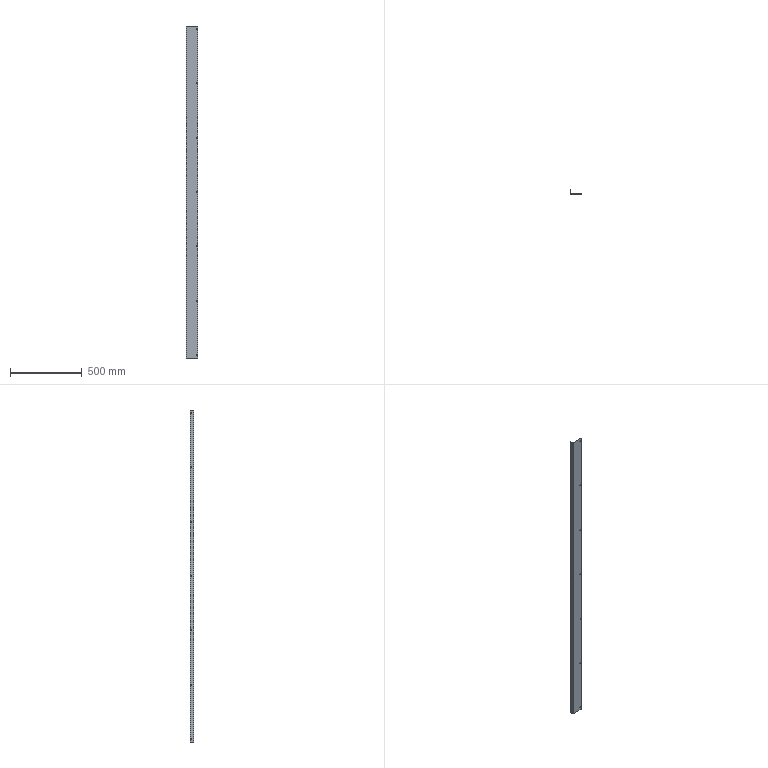Part | 1 solid | 70 faces | box 79 x 24 x 2316 mm | volume 234888 mm3 | plane 40 | cylinder 30 | commonest cylinder face diameters 6 x28 0.4 x1 2.4 x1